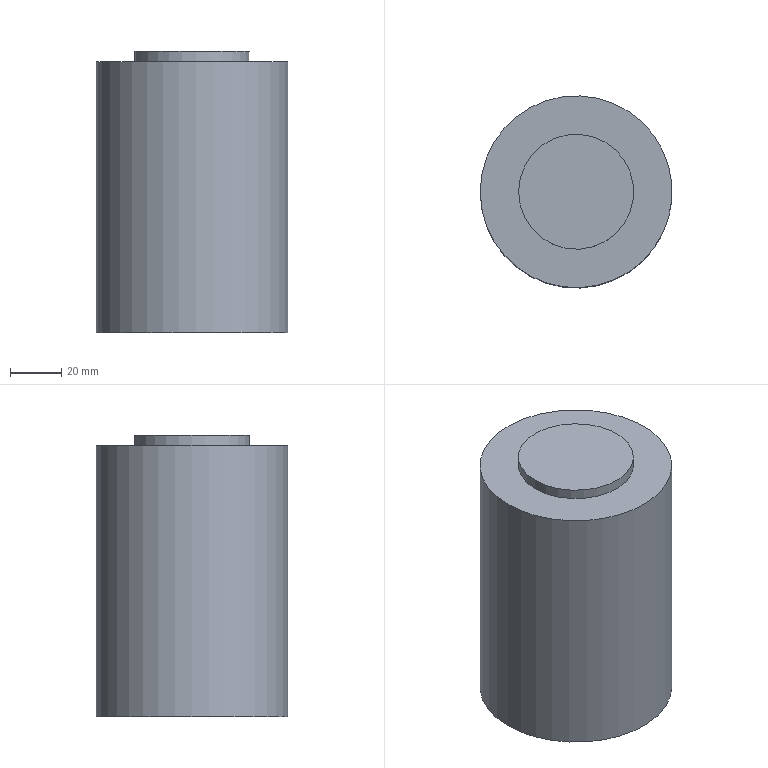Part | NX | features solid 2 | 1 solid | 5 faces | box 75 x 75 x 110 mm | volume 474655 mm3 | plane 3 | cylinder 2 | commonest cylinder face diameters 45 x1 75 x1
STEP:
#1=CARTESIAN_POINT('',(1272.5,-830.,-49.));
#2=VERTEX_POINT('',#1);
#3=CARTESIAN_POINT('',(1295.,-830.,-49.));
#4=DIRECTION('',(0.,0.,-1.));
#5=DIRECTION('',(-1.,0.,0.));
#6=AXIS2_PLACEMENT_3D('',#3,#4,#5);
#7=CIRCLE('',#6,22.5);
#8=EDGE_CURVE('',#2,#2,#7,.F.);
#9=ORIENTED_EDGE('',*,*,#8,.F.);
#10=EDGE_LOOP('',(#9));
#11=FACE_BOUND('',#10,.T.);
#12=CARTESIAN_POINT('',(1257.5,-830.,-49.));
#13=VERTEX_POINT('',#12);
#14=CARTESIAN_POINT('',(1295.,-830.,-49.));
#15=DIRECTION('',(0.,0.,-1.));
#16=DIRECTION('',(-1.,0.,0.));
#17=AXIS2_PLACEMENT_3D('',#14,#15,#16);
#18=CIRCLE('',#17,37.5);
#19=EDGE_CURVE('',#13,#13,#18,.T.);
#20=ORIENTED_EDGE('',*,*,#19,.F.);
#21=EDGE_LOOP('',(#20));
#22=FACE_BOUND('',#21,.T.);
#23=CARTESIAN_POINT('',(1295.,-830.,-49.));
#24=DIRECTION('',(0.,0.,1.));
#25=DIRECTION('',(1.,0.,0.));
#26=AXIS2_PLACEMENT_3D('',#23,#24,#25);
#27=PLANE('',#26);
#28=ADVANCED_FACE('',(#11,#22),#27,.T.);
#29=CARTESIAN_POINT('',(1257.5,-830.,-155.));
#30=VERTEX_POINT('',#29);
#31=CARTESIAN_POINT('',(1295.,-830.,-155.));
#32=DIRECTION('',(0.,0.,-1.));
#33=DIRECTION('',(-1.,0.,0.));
#34=AXIS2_PLACEMENT_3D('',#31,#32,#33);
#35=CIRCLE('',#34,37.5);
#36=EDGE_CURVE('',#30,#30,#35,.F.);
#37=ORIENTED_EDGE('',*,*,#36,.F.);
#38=EDGE_LOOP('',(#37));
#39=FACE_BOUND('',#38,.T.);
#40=CARTESIAN_POINT('',(1335.,-893.5,-155.));
#41=DIRECTION('',(0.,0.,-1.));
#42=DIRECTION('',(-1.,0.,0.));
#43=AXIS2_PLACEMENT_3D('',#40,#41,#42);
#44=PLANE('',#43);
#45=ADVANCED_FACE('',(#39),#44,.T.);
#46=ORIENTED_EDGE('',*,*,#19,.T.);
#47=EDGE_LOOP('',(#46));
#48=FACE_BOUND('',#47,.T.);
#49=ORIENTED_EDGE('',*,*,#36,.T.);
#50=EDGE_LOOP('',(#49));
#51=FACE_BOUND('',#50,.T.);
#52=CARTESIAN_POINT('',(1295.,-830.,-64.));
#53=DIRECTION('',(0.,0.,1.));
#54=DIRECTION('',(1.,0.,0.));
#55=AXIS2_PLACEMENT_3D('',#52,#53,#54);
#56=CYLINDRICAL_SURFACE('',#55,37.5);
#57=ADVANCED_FACE('',(#48,#51),#56,.T.);
#58=CARTESIAN_POINT('',(1272.5,-830.,-45.));
#59=VERTEX_POINT('',#58);
#60=CARTESIAN_POINT('',(1295.,-830.,-45.));
#61=DIRECTION('',(0.,0.,-1.));
#62=DIRECTION('',(-1.,0.,0.));
#63=AXIS2_PLACEMENT_3D('',#60,#61,#62);
#64=CIRCLE('',#63,22.5);
#65=EDGE_CURVE('',#59,#59,#64,.F.);
#66=ORIENTED_EDGE('',*,*,#65,.T.);
#67=EDGE_LOOP('',(#66));
#68=FACE_BOUND('',#67,.T.);
#69=CARTESIAN_POINT('',(1295.,-830.,-45.));
#70=DIRECTION('',(0.,0.,1.));
#71=DIRECTION('',(1.,0.,0.));
#72=AXIS2_PLACEMENT_3D('',#69,#70,#71);
#73=PLANE('',#72);
#74=ADVANCED_FACE('',(#68),#73,.T.);
#75=ORIENTED_EDGE('',*,*,#65,.F.);
#76=EDGE_LOOP('',(#75));
#77=FACE_BOUND('',#76,.T.);
#78=ORIENTED_EDGE('',*,*,#8,.T.);
#79=EDGE_LOOP('',(#78));
#80=FACE_BOUND('',#79,.T.);
#81=CARTESIAN_POINT('',(1295.,-830.,-63.));
#82=DIRECTION('',(0.,0.,1.));
#83=DIRECTION('',(1.,0.,0.));
#84=AXIS2_PLACEMENT_3D('',#81,#82,#83);
#85=CYLINDRICAL_SURFACE('',#84,22.5);
#86=ADVANCED_FACE('',(#77,#80),#85,.T.);
#87=CLOSED_SHELL('',(#28,#45,#57,#74,#86));
#88=MANIFOLD_SOLID_BREP('',#87);
#89=(LENGTH_UNIT()NAMED_UNIT(*)SI_UNIT(.MILLI.,.METRE.));
#90=UNCERTAINTY_MEASURE_WITH_UNIT(LENGTH_MEASURE(0.00001),#89,'','');
#91=(NAMED_UNIT(*)PLANE_ANGLE_UNIT()SI_UNIT($,.RADIAN.));
#92=(NAMED_UNIT(*)SI_UNIT($,.STERADIAN.)SOLID_ANGLE_UNIT());
#93=(GEOMETRIC_REPRESENTATION_CONTEXT(3)GLOBAL_UNCERTAINTY_ASSIGNED_CONTEXT((#90))GLOBAL_UNIT_ASSIGNED_CONTEXT((#89,#91,#92))REPRESENTATION_CONTEXT('',''));
#94=ADVANCED_BREP_SHAPE_REPRESENTATION('',(#88),#93);